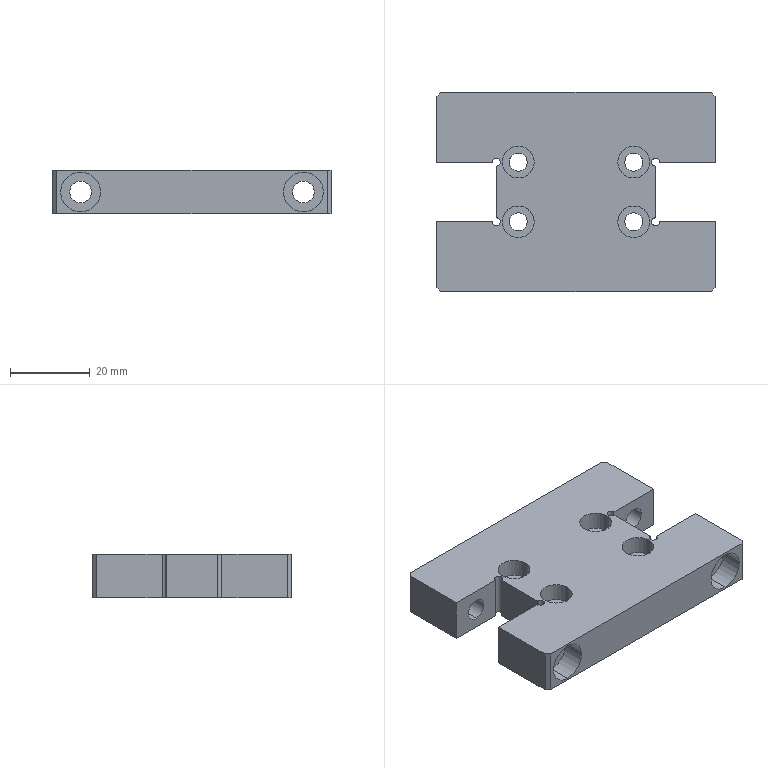Part | SolidWorks | features BaseBody 1 | 1 solid | 64 faces | box 70 x 50 x 11 mm | volume 29180 mm3 | cylinder 38 | plane 26 | commonest cylinder face diameters 4.5 x8 5.5 x8 8 x8 10 x8 2 x6